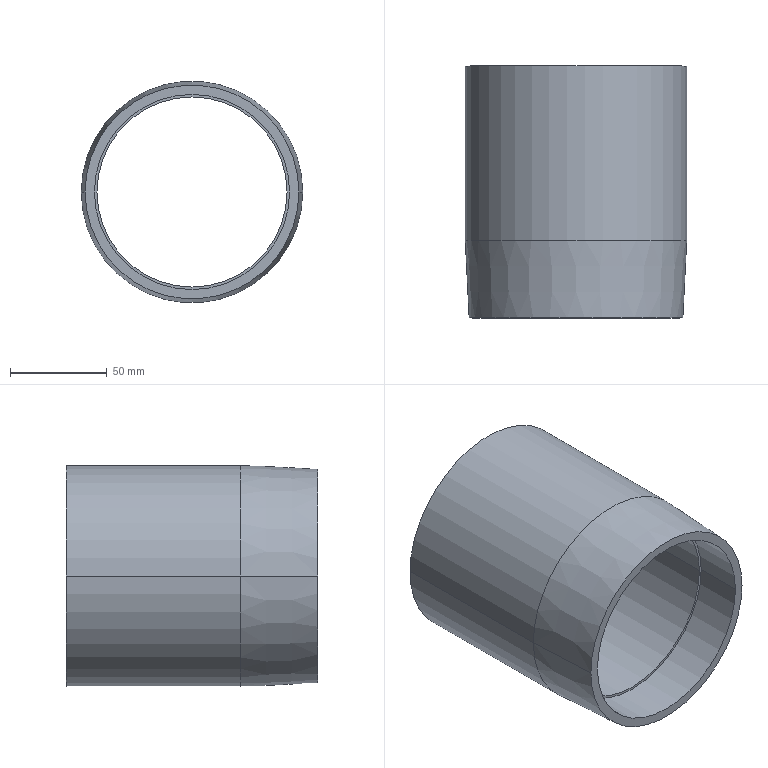Part | STEP file | ROLLER.2.stp | 1 solid | 14 faces | box 114.3 x 130 x 114.3 mm | volume 316826 mm3 | cylinder 8 | plane 4 | cone 2 | commonest cylinder face diameters 100.7 x4 98.1 x2 114.3 x2
STEP:
#1=CARTESIAN_POINT('',(0.,0.,0.));
#2=DIRECTION('',(0.,0.,1.));
#3=DIRECTION('',(1.,0.,0.));
#4=AXIS2_PLACEMENT_3D('',#1,#2,#3);
#5=CARTESIAN_POINT('',(49.05,40.,0.));
#6=VERTEX_POINT('',#5);
#7=CARTESIAN_POINT('',(-49.05,40.,0.));
#8=VERTEX_POINT('',#7);
#9=CARTESIAN_POINT('',(0.,40.,0.));
#10=DIRECTION('',(0.,1.,0.));
#11=DIRECTION('',(1.,0.,0.));
#12=AXIS2_PLACEMENT_3D('',#9,#10,#11);
#13=CIRCLE('',#12,49.05);
#14=CARTESIAN_POINT('',(49.7,40.,0.));
#15=DIRECTION('',(0.,1.,0.));
#16=DIRECTION('',(1.,0.,0.));
#17=AXIS2_PLACEMENT_3D('',#14,#15,#16);
#18=PLANE('',#17);
#19=CARTESIAN_POINT('',(-49.7,0.));
#20=DIRECTION('',(1.,0.));
#21=AXIS2_PLACEMENT_2D('',#19,#20);
#22=CIRCLE('',#21,49.05);
#23=(GEOMETRIC_REPRESENTATION_CONTEXT(2)PARAMETRIC_REPRESENTATION_CONTEXT()REPRESENTATION_CONTEXT('',''));
#24=DEFINITIONAL_REPRESENTATION('',(#22),#23);
#25=PCURVE('',#18,#24);
#26=CARTESIAN_POINT('',(0.,-2.5,0.));
#27=DIRECTION('',(0.,1.,0.));
#28=DIRECTION('',(1.,0.,0.));
#29=AXIS2_PLACEMENT_3D('',#26,#27,#28);
#30=CYLINDRICAL_SURFACE('',#29,49.05);
#31=CARTESIAN_POINT('',(0.,42.5));
#32=DIRECTION('',(1.,0.));
#33=VECTOR('',#32,1.);
#34=LINE('',#31,#33);
#35=(GEOMETRIC_REPRESENTATION_CONTEXT(2)PARAMETRIC_REPRESENTATION_CONTEXT()REPRESENTATION_CONTEXT('',''));
#36=DEFINITIONAL_REPRESENTATION('',(#34),#35);
#37=PCURVE('',#30,#36);
#38=SURFACE_CURVE('',#13,(#25,#37),.PCURVE_S1.);
#39=EDGE_CURVE('',#6,#8,#38,.T.);
#40=ORIENTED_EDGE('',*,*,#39,.F.);
#41=CARTESIAN_POINT('',(0.,40.,0.));
#42=DIRECTION('',(0.,1.,0.));
#43=DIRECTION('',(1.,0.,0.));
#44=AXIS2_PLACEMENT_3D('',#41,#42,#43);
#45=CIRCLE('',#44,49.05);
#46=CARTESIAN_POINT('',(-49.7,0.));
#47=DIRECTION('',(1.,0.));
#48=AXIS2_PLACEMENT_2D('',#46,#47);
#49=CIRCLE('',#48,49.05);
#50=(GEOMETRIC_REPRESENTATION_CONTEXT(2)PARAMETRIC_REPRESENTATION_CONTEXT()REPRESENTATION_CONTEXT('',''));
#51=DEFINITIONAL_REPRESENTATION('',(#49),#50);
#52=PCURVE('',#18,#51);
#53=CARTESIAN_POINT('',(0.,-2.5,0.));
#54=DIRECTION('',(0.,1.,0.));
#55=DIRECTION('',(1.,0.,0.));
#56=AXIS2_PLACEMENT_3D('',#53,#54,#55);
#57=CYLINDRICAL_SURFACE('',#56,49.05);
#58=CARTESIAN_POINT('',(0.,42.5));
#59=DIRECTION('',(1.,0.));
#60=VECTOR('',#59,1.);
#61=LINE('',#58,#60);
#62=(GEOMETRIC_REPRESENTATION_CONTEXT(2)PARAMETRIC_REPRESENTATION_CONTEXT()REPRESENTATION_CONTEXT('',''));
#63=DEFINITIONAL_REPRESENTATION('',(#61),#62);
#64=PCURVE('',#57,#63);
#65=SURFACE_CURVE('',#45,(#52,#64),.PCURVE_S1.);
#66=EDGE_CURVE('',#8,#6,#65,.T.);
#67=ORIENTED_EDGE('',*,*,#66,.F.);
#68=EDGE_LOOP('',(#40,#67));
#69=FACE_BOUND('',#68,.T.);
#70=CARTESIAN_POINT('',(50.35,40.,0.));
#71=VERTEX_POINT('',#70);
#72=CARTESIAN_POINT('',(-50.35,40.,0.));
#73=VERTEX_POINT('',#72);
#74=CARTESIAN_POINT('',(0.,40.,0.));
#75=DIRECTION('',(0.,1.,0.));
#76=DIRECTION('',(1.,0.,0.));
#77=AXIS2_PLACEMENT_3D('',#74,#75,#76);
#78=CIRCLE('',#77,50.35);
#79=CARTESIAN_POINT('',(-49.7,0.));
#80=DIRECTION('',(1.,0.));
#81=AXIS2_PLACEMENT_2D('',#79,#80);
#82=CIRCLE('',#81,50.35);
#83=(GEOMETRIC_REPRESENTATION_CONTEXT(2)PARAMETRIC_REPRESENTATION_CONTEXT()REPRESENTATION_CONTEXT('',''));
#84=DEFINITIONAL_REPRESENTATION('',(#82),#83);
#85=PCURVE('',#18,#84);
#86=CARTESIAN_POINT('',(0.,50.,0.));
#87=DIRECTION('',(0.,1.,0.));
#88=DIRECTION('',(1.,0.,0.));
#89=AXIS2_PLACEMENT_3D('',#86,#87,#88);
#90=CYLINDRICAL_SURFACE('',#89,50.35);
#91=CARTESIAN_POINT('',(0.,-10.));
#92=DIRECTION('',(1.,0.));
#93=VECTOR('',#92,1.);
#94=LINE('',#91,#93);
#95=(GEOMETRIC_REPRESENTATION_CONTEXT(2)PARAMETRIC_REPRESENTATION_CONTEXT()REPRESENTATION_CONTEXT('',''));
#96=DEFINITIONAL_REPRESENTATION('',(#94),#95);
#97=PCURVE('',#90,#96);
#98=SURFACE_CURVE('',#78,(#85,#97),.PCURVE_S1.);
#99=EDGE_CURVE('',#71,#73,#98,.T.);
#100=ORIENTED_EDGE('',*,*,#99,.T.);
#101=CARTESIAN_POINT('',(0.,40.,0.));
#102=DIRECTION('',(0.,1.,0.));
#103=DIRECTION('',(1.,0.,0.));
#104=AXIS2_PLACEMENT_3D('',#101,#102,#103);
#105=CIRCLE('',#104,50.35);
#106=CARTESIAN_POINT('',(-49.7,0.));
#107=DIRECTION('',(1.,0.));
#108=AXIS2_PLACEMENT_2D('',#106,#107);
#109=CIRCLE('',#108,50.35);
#110=(GEOMETRIC_REPRESENTATION_CONTEXT(2)PARAMETRIC_REPRESENTATION_CONTEXT()REPRESENTATION_CONTEXT('',''));
#111=DEFINITIONAL_REPRESENTATION('',(#109),#110);
#112=PCURVE('',#18,#111);
#113=CARTESIAN_POINT('',(0.,50.,0.));
#114=DIRECTION('',(0.,1.,0.));
#115=DIRECTION('',(1.,0.,0.));
#116=AXIS2_PLACEMENT_3D('',#113,#114,#115);
#117=CYLINDRICAL_SURFACE('',#116,50.35);
#118=CARTESIAN_POINT('',(0.,-10.));
#119=DIRECTION('',(1.,0.));
#120=VECTOR('',#119,1.);
#121=LINE('',#118,#120);
#122=(GEOMETRIC_REPRESENTATION_CONTEXT(2)PARAMETRIC_REPRESENTATION_CONTEXT()REPRESENTATION_CONTEXT('',''));
#123=DEFINITIONAL_REPRESENTATION('',(#121),#122);
#124=PCURVE('',#117,#123);
#125=SURFACE_CURVE('',#105,(#112,#124),.PCURVE_S1.);
#126=EDGE_CURVE('',#73,#71,#125,.T.);
#127=ORIENTED_EDGE('',*,*,#126,.T.);
#128=EDGE_LOOP('',(#100,#127));
#129=FACE_BOUND('',#128,.T.);
#130=ADVANCED_FACE('',(#69,#129),#18,.T.);
#131=CARTESIAN_POINT('',(50.35,65.,0.));
#132=VERTEX_POINT('',#131);
#133=CARTESIAN_POINT('',(-50.35,65.,0.));
#134=VERTEX_POINT('',#133);
#135=CARTESIAN_POINT('',(0.,65.,0.));
#136=DIRECTION('',(0.,1.,0.));
#137=DIRECTION('',(1.,0.,0.));
#138=AXIS2_PLACEMENT_3D('',#135,#136,#137);
#139=CIRCLE('',#138,50.35);
#140=CARTESIAN_POINT('',(53.75,65.,0.));
#141=DIRECTION('',(0.,1.,0.));
#142=DIRECTION('',(1.,0.,0.));
#143=AXIS2_PLACEMENT_3D('',#140,#141,#142);
#144=PLANE('',#143);
#145=CARTESIAN_POINT('',(-53.75,0.));
#146=DIRECTION('',(1.,0.));
#147=AXIS2_PLACEMENT_2D('',#145,#146);
#148=CIRCLE('',#147,50.35);
#149=(GEOMETRIC_REPRESENTATION_CONTEXT(2)PARAMETRIC_REPRESENTATION_CONTEXT()REPRESENTATION_CONTEXT('',''));
#150=DEFINITIONAL_REPRESENTATION('',(#148),#149);
#151=PCURVE('',#144,#150);
#152=CARTESIAN_POINT('',(0.,15.));
#153=DIRECTION('',(1.,0.));
#154=VECTOR('',#153,1.);
#155=LINE('',#152,#154);
#156=(GEOMETRIC_REPRESENTATION_CONTEXT(2)PARAMETRIC_REPRESENTATION_CONTEXT()REPRESENTATION_CONTEXT('',''));
#157=DEFINITIONAL_REPRESENTATION('',(#155),#156);
#158=PCURVE('',#90,#157);
#159=SURFACE_CURVE('',#139,(#151,#158),.PCURVE_S1.);
#160=EDGE_CURVE('',#132,#134,#159,.T.);
#161=ORIENTED_EDGE('',*,*,#160,.F.);
#162=CARTESIAN_POINT('',(0.,65.,0.));
#163=DIRECTION('',(0.,1.,0.));
#164=DIRECTION('',(1.,0.,0.));
#165=AXIS2_PLACEMENT_3D('',#162,#163,#164);
#166=CIRCLE('',#165,50.35);
#167=CARTESIAN_POINT('',(-53.75,0.));
#168=DIRECTION('',(1.,0.));
#169=AXIS2_PLACEMENT_2D('',#167,#168);
#170=CIRCLE('',#169,50.35);
#171=(GEOMETRIC_REPRESENTATION_CONTEXT(2)PARAMETRIC_REPRESENTATION_CONTEXT()REPRESENTATION_CONTEXT('',''));
#172=DEFINITIONAL_REPRESENTATION('',(#170),#171);
#173=PCURVE('',#144,#172);
#174=CARTESIAN_POINT('',(0.,15.));
#175=DIRECTION('',(1.,0.));
#176=VECTOR('',#175,1.);
#177=LINE('',#174,#176);
#178=(GEOMETRIC_REPRESENTATION_CONTEXT(2)PARAMETRIC_REPRESENTATION_CONTEXT()REPRESENTATION_CONTEXT('',''));
#179=DEFINITIONAL_REPRESENTATION('',(#177),#178);
#180=PCURVE('',#117,#179);
#181=SURFACE_CURVE('',#166,(#173,#180),.PCURVE_S1.);
#182=EDGE_CURVE('',#134,#132,#181,.T.);
#183=ORIENTED_EDGE('',*,*,#182,.F.);
#184=EDGE_LOOP('',(#161,#183));
#185=FACE_BOUND('',#184,.T.);
#186=CARTESIAN_POINT('',(57.15,65.,0.));
#187=VERTEX_POINT('',#186);
#188=CARTESIAN_POINT('',(-57.15,65.,0.));
#189=VERTEX_POINT('',#188);
#190=CARTESIAN_POINT('',(0.,65.,0.));
#191=DIRECTION('',(0.,1.,0.));
#192=DIRECTION('',(1.,0.,0.));
#193=AXIS2_PLACEMENT_3D('',#190,#191,#192);
#194=CIRCLE('',#193,57.15);
#195=CARTESIAN_POINT('',(-53.75,0.));
#196=DIRECTION('',(1.,0.));
#197=AXIS2_PLACEMENT_2D('',#195,#196);
#198=CIRCLE('',#197,57.15);
#199=(GEOMETRIC_REPRESENTATION_CONTEXT(2)PARAMETRIC_REPRESENTATION_CONTEXT()REPRESENTATION_CONTEXT('',''));
#200=DEFINITIONAL_REPRESENTATION('',(#198),#199);
#201=PCURVE('',#144,#200);
#202=CARTESIAN_POINT('',(0.,20.,0.));
#203=DIRECTION('',(0.,1.,0.));
#204=DIRECTION('',(1.,0.,0.));
#205=AXIS2_PLACEMENT_3D('',#202,#203,#204);
#206=CYLINDRICAL_SURFACE('',#205,57.15);
#207=CARTESIAN_POINT('',(0.,45.));
#208=DIRECTION('',(1.,0.));
#209=VECTOR('',#208,1.);
#210=LINE('',#207,#209);
#211=(GEOMETRIC_REPRESENTATION_CONTEXT(2)PARAMETRIC_REPRESENTATION_CONTEXT()REPRESENTATION_CONTEXT('',''));
#212=DEFINITIONAL_REPRESENTATION('',(#210),#211);
#213=PCURVE('',#206,#212);
#214=SURFACE_CURVE('',#194,(#201,#213),.PCURVE_S1.);
#215=EDGE_CURVE('',#187,#189,#214,.T.);
#216=ORIENTED_EDGE('',*,*,#215,.T.);
#217=CARTESIAN_POINT('',(0.,65.,0.));
#218=DIRECTION('',(0.,1.,0.));
#219=DIRECTION('',(1.,0.,0.));
#220=AXIS2_PLACEMENT_3D('',#217,#218,#219);
#221=CIRCLE('',#220,57.15);
#222=CARTESIAN_POINT('',(-53.75,0.));
#223=DIRECTION('',(1.,0.));
#224=AXIS2_PLACEMENT_2D('',#222,#223);
#225=CIRCLE('',#224,57.15);
#226=(GEOMETRIC_REPRESENTATION_CONTEXT(2)PARAMETRIC_REPRESENTATION_CONTEXT()REPRESENTATION_CONTEXT('',''));
#227=DEFINITIONAL_REPRESENTATION('',(#225),#226);
#228=PCURVE('',#144,#227);
#229=CARTESIAN_POINT('',(0.,20.,0.));
#230=DIRECTION('',(0.,1.,0.));
#231=DIRECTION('',(1.,0.,0.));
#232=AXIS2_PLACEMENT_3D('',#229,#230,#231);
#233=CYLINDRICAL_SURFACE('',#232,57.15);
#234=CARTESIAN_POINT('',(0.,45.));
#235=DIRECTION('',(1.,0.));
#236=VECTOR('',#235,1.);
#237=LINE('',#234,#236);
#238=(GEOMETRIC_REPRESENTATION_CONTEXT(2)PARAMETRIC_REPRESENTATION_CONTEXT()REPRESENTATION_CONTEXT('',''));
#239=DEFINITIONAL_REPRESENTATION('',(#237),#238);
#240=PCURVE('',#233,#239);
#241=SURFACE_CURVE('',#221,(#228,#240),.PCURVE_S1.);
#242=EDGE_CURVE('',#189,#187,#241,.T.);
#243=ORIENTED_EDGE('',*,*,#242,.T.);
#244=EDGE_LOOP('',(#216,#243));
#245=FACE_BOUND('',#244,.T.);
#246=ADVANCED_FACE('',(#185,#245),#144,.T.);
#247=CARTESIAN_POINT('',(57.15,-25.,0.));
#248=VERTEX_POINT('',#247);
#249=CARTESIAN_POINT('',(57.15,65.,0.));
#250=DIRECTION('',(0.,-1.,0.));
#251=VECTOR('',#250,1.);
#252=LINE('',#249,#251);
#253=CARTESIAN_POINT('',(0.,45.));
#254=DIRECTION('',(0.,-1.));
#255=VECTOR('',#254,1.);
#256=LINE('',#253,#255);
#257=(GEOMETRIC_REPRESENTATION_CONTEXT(2)PARAMETRIC_REPRESENTATION_CONTEXT()REPRESENTATION_CONTEXT('',''));
#258=DEFINITIONAL_REPRESENTATION('',(#256),#257);
#259=PCURVE('',#206,#258);
#260=CARTESIAN_POINT('',(6.283,45.));
#261=DIRECTION('',(0.,-1.));
#262=VECTOR('',#261,1.);
#263=LINE('',#260,#262);
#264=(GEOMETRIC_REPRESENTATION_CONTEXT(2)PARAMETRIC_REPRESENTATION_CONTEXT()REPRESENTATION_CONTEXT('',''));
#265=DEFINITIONAL_REPRESENTATION('',(#263),#264);
#266=PCURVE('',#233,#265);
#267=SURFACE_CURVE('',#252,(#259,#266),.PCURVE_S1.);
#268=EDGE_CURVE('',#187,#248,#267,.T.);
#269=ORIENTED_EDGE('',*,*,#268,.T.);
#270=CARTESIAN_POINT('',(-57.15,-25.,0.));
#271=VERTEX_POINT('',#270);
#272=CARTESIAN_POINT('',(0.,-25.,0.));
#273=DIRECTION('',(0.,1.,0.));
#274=DIRECTION('',(1.,0.,0.));
#275=AXIS2_PLACEMENT_3D('',#272,#273,#274);
#276=CIRCLE('',#275,57.15);
#277=CARTESIAN_POINT('',(0.,-45.));
#278=DIRECTION('',(1.,0.));
#279=VECTOR('',#278,1.);
#280=LINE('',#277,#279);
#281=(GEOMETRIC_REPRESENTATION_CONTEXT(2)PARAMETRIC_REPRESENTATION_CONTEXT()REPRESENTATION_CONTEXT('',''));
#282=DEFINITIONAL_REPRESENTATION('',(#280),#281);
#283=PCURVE('',#206,#282);
#284=CARTESIAN_POINT('',(0.,-45.,0.));
#285=DIRECTION('',(0.,1.,0.));
#286=DIRECTION('',(1.,0.,0.));
#287=AXIS2_PLACEMENT_3D('',#284,#285,#286);
#288=CONICAL_SURFACE('',#287,56.15,0.04996);
#289=CARTESIAN_POINT('',(0.,20.));
#290=DIRECTION('',(1.,0.));
#291=VECTOR('',#290,1.);
#292=LINE('',#289,#291);
#293=(GEOMETRIC_REPRESENTATION_CONTEXT(2)PARAMETRIC_REPRESENTATION_CONTEXT()REPRESENTATION_CONTEXT('',''));
#294=DEFINITIONAL_REPRESENTATION('',(#292),#293);
#295=PCURVE('',#288,#294);
#296=SURFACE_CURVE('',#276,(#283,#295),.PCURVE_S1.);
#297=EDGE_CURVE('',#248,#271,#296,.T.);
#298=ORIENTED_EDGE('',*,*,#297,.T.);
#299=CARTESIAN_POINT('',(-57.15,65.,0.));
#300=DIRECTION('',(0.,-1.,0.));
#301=VECTOR('',#300,1.);
#302=LINE('',#299,#301);
#303=CARTESIAN_POINT('',(3.142,45.));
#304=DIRECTION('',(0.,-1.));
#305=VECTOR('',#304,1.);
#306=LINE('',#303,#305);
#307=(GEOMETRIC_REPRESENTATION_CONTEXT(2)PARAMETRIC_REPRESENTATION_CONTEXT()REPRESENTATION_CONTEXT('',''));
#308=DEFINITIONAL_REPRESENTATION('',(#306),#307);
#309=PCURVE('',#206,#308);
#310=CARTESIAN_POINT('',(3.142,45.));
#311=DIRECTION('',(0.,-1.));
#312=VECTOR('',#311,1.);
#313=LINE('',#310,#312);
#314=(GEOMETRIC_REPRESENTATION_CONTEXT(2)PARAMETRIC_REPRESENTATION_CONTEXT()REPRESENTATION_CONTEXT('',''));
#315=DEFINITIONAL_REPRESENTATION('',(#313),#314);
#316=PCURVE('',#233,#315);
#317=SURFACE_CURVE('',#302,(#309,#316),.PCURVE_S1.);
#318=EDGE_CURVE('',#189,#271,#317,.T.);
#319=ORIENTED_EDGE('',*,*,#318,.F.);
#320=ORIENTED_EDGE('',*,*,#215,.F.);
#321=EDGE_LOOP('',(#269,#298,#319,#320));
#322=FACE_BOUND('',#321,.T.);
#323=ADVANCED_FACE('',(#322),#206,.T.);
#324=CARTESIAN_POINT('',(55.15,-65.,0.));
#325=VERTEX_POINT('',#324);
#326=CARTESIAN_POINT('',(57.15,-25.,0.));
#327=DIRECTION('',(-0.04994,-0.9988,0.));
#328=VECTOR('',#327,1.);
#329=LINE('',#326,#328);
#330=CARTESIAN_POINT('',(0.,20.));
#331=DIRECTION('',(0.,-1.));
#332=VECTOR('',#331,1.);
#333=LINE('',#330,#332);
#334=(GEOMETRIC_REPRESENTATION_CONTEXT(2)PARAMETRIC_REPRESENTATION_CONTEXT()REPRESENTATION_CONTEXT('',''));
#335=DEFINITIONAL_REPRESENTATION('',(#333),#334);
#336=PCURVE('',#288,#335);
#337=CARTESIAN_POINT('',(0.,-45.,0.));
#338=DIRECTION('',(0.,1.,0.));
#339=DIRECTION('',(1.,0.,0.));
#340=AXIS2_PLACEMENT_3D('',#337,#338,#339);
#341=CONICAL_SURFACE('',#340,56.15,0.04996);
#342=CARTESIAN_POINT('',(6.283,20.));
#343=DIRECTION('',(0.,-1.));
#344=VECTOR('',#343,1.);
#345=LINE('',#342,#344);
#346=(GEOMETRIC_REPRESENTATION_CONTEXT(2)PARAMETRIC_REPRESENTATION_CONTEXT()REPRESENTATION_CONTEXT('',''));
#347=DEFINITIONAL_REPRESENTATION('',(#345),#346);
#348=PCURVE('',#341,#347);
#349=SURFACE_CURVE('',#329,(#336,#348),.PCURVE_S1.);
#350=EDGE_CURVE('',#248,#325,#349,.T.);
#351=ORIENTED_EDGE('',*,*,#350,.T.);
#352=CARTESIAN_POINT('',(-55.15,-65.,0.));
#353=VERTEX_POINT('',#352);
#354=CARTESIAN_POINT('',(0.,-65.,0.));
#355=DIRECTION('',(0.,1.,0.));
#356=DIRECTION('',(1.,0.,0.));
#357=AXIS2_PLACEMENT_3D('',#354,#355,#356);
#358=CIRCLE('',#357,55.15);
#359=CARTESIAN_POINT('',(0.,-20.));
#360=DIRECTION('',(1.,0.));
#361=VECTOR('',#360,1.);
#362=LINE('',#359,#361);
#363=(GEOMETRIC_REPRESENTATION_CONTEXT(2)PARAMETRIC_REPRESENTATION_CONTEXT()REPRESENTATION_CONTEXT('',''));
#364=DEFINITIONAL_REPRESENTATION('',(#362),#363);
#365=PCURVE('',#288,#364);
#366=CARTESIAN_POINT('',(52.75,-65.,0.));
#367=DIRECTION('',(0.,-1.,0.));
#368=DIRECTION('',(0.,0.,-1.));
#369=AXIS2_PLACEMENT_3D('',#366,#367,#368);
#370=PLANE('',#369);
#371=CARTESIAN_POINT('',(0.,2.4));
#372=CARTESIAN_POINT('',(95.523,2.4));
#373=CARTESIAN_POINT('',(47.761,-80.325));
#374=CARTESIAN_POINT('',(0.,-163.05));
#375=CARTESIAN_POINT('',(-47.761,-80.325));
#376=CARTESIAN_POINT('',(-95.523,2.4));
#377=CARTESIAN_POINT('',(0.,2.4));
#378=(BOUNDED_CURVE()B_SPLINE_CURVE(2,(#371,#372,#373,#374,#375,#376,#377),.UNSPECIFIED.,.T.,.F.)B_SPLINE_CURVE_WITH_KNOTS((1,2,2,2,2,1),(-2.094,0.,2.094,4.189,6.283,8.378),.UNSPECIFIED.)CURVE()GEOMETRIC_REPRESENTATION_ITEM()RATIONAL_B_SPLINE_CURVE((1.,0.5,1.,0.5,1.,0.5,1.))REPRESENTATION_ITEM(''));
#379=(GEOMETRIC_REPRESENTATION_CONTEXT(2)PARAMETRIC_REPRESENTATION_CONTEXT()REPRESENTATION_CONTEXT('',''));
#380=DEFINITIONAL_REPRESENTATION('',(#378),#379);
#381=PCURVE('',#370,#380);
#382=SURFACE_CURVE('',#358,(#365,#381),.PCURVE_S1.);
#383=EDGE_CURVE('',#325,#353,#382,.T.);
#384=ORIENTED_EDGE('',*,*,#383,.T.);
#385=CARTESIAN_POINT('',(-57.15,-25.,0.));
#386=DIRECTION('',(0.04994,-0.9988,0.));
#387=VECTOR('',#386,1.);
#388=LINE('',#385,#387);
#389=CARTESIAN_POINT('',(3.142,20.));
#390=DIRECTION('',(0.,-1.));
#391=VECTOR('',#390,1.);
#392=LINE('',#389,#391);
#393=(GEOMETRIC_REPRESENTATION_CONTEXT(2)PARAMETRIC_REPRESENTATION_CONTEXT()REPRESENTATION_CONTEXT('',''));
#394=DEFINITIONAL_REPRESENTATION('',(#392),#393);
#395=PCURVE('',#288,#394);
#396=CARTESIAN_POINT('',(3.142,20.));
#397=DIRECTION('',(0.,-1.));
#398=VECTOR('',#397,1.);
#399=LINE('',#396,#398);
#400=(GEOMETRIC_REPRESENTATION_CONTEXT(2)PARAMETRIC_REPRESENTATION_CONTEXT()REPRESENTATION_CONTEXT('',''));
#401=DEFINITIONAL_REPRESENTATION('',(#399),#400);
#402=PCURVE('',#341,#401);
#403=SURFACE_CURVE('',#388,(#395,#402),.PCURVE_S1.);
#404=EDGE_CURVE('',#271,#353,#403,.T.);
#405=ORIENTED_EDGE('',*,*,#404,.F.);
#406=ORIENTED_EDGE('',*,*,#297,.F.);
#407=EDGE_LOOP('',(#351,#384,#405,#406));
#408=FACE_BOUND('',#407,.T.);
#409=ADVANCED_FACE('',(#408),#288,.T.);
#410=CARTESIAN_POINT('',(50.35,-65.,0.));
#411=VERTEX_POINT('',#410);
#412=CARTESIAN_POINT('',(-50.35,-65.,0.));
#413=VERTEX_POINT('',#412);
#414=CARTESIAN_POINT('',(0.,-65.,0.));
#415=DIRECTION('',(0.,1.,0.));
#416=DIRECTION('',(1.,0.,0.));
#417=AXIS2_PLACEMENT_3D('',#414,#415,#416);
#418=CIRCLE('',#417,50.35);
#419=CARTESIAN_POINT('',(0.,-2.4));
#420=CARTESIAN_POINT('',(87.209,-2.4));
#421=CARTESIAN_POINT('',(43.604,-77.925));
#422=CARTESIAN_POINT('',(0.,-153.45));
#423=CARTESIAN_POINT('',(-43.604,-77.925));
#424=CARTESIAN_POINT('',(-87.209,-2.4));
#425=CARTESIAN_POINT('',(0.,-2.4));
#426=(BOUNDED_CURVE()B_SPLINE_CURVE(2,(#419,#420,#421,#422,#423,#424,#425),.UNSPECIFIED.,.T.,.F.)B_SPLINE_CURVE_WITH_KNOTS((1,2,2,2,2,1),(-2.094,0.,2.094,4.189,6.283,8.378),.UNSPECIFIED.)CURVE()GEOMETRIC_REPRESENTATION_ITEM()RATIONAL_B_SPLINE_CURVE((1.,0.5,1.,0.5,1.,0.5,1.))REPRESENTATION_ITEM(''));
#427=(GEOMETRIC_REPRESENTATION_CONTEXT(2)PARAMETRIC_REPRESENTATION_CONTEXT()REPRESENTATION_CONTEXT('',''));
#428=DEFINITIONAL_REPRESENTATION('',(#426),#427);
#429=PCURVE('',#370,#428);
#430=CARTESIAN_POINT('',(0.,-52.5,0.));
#431=DIRECTION('',(0.,1.,0.));
#432=DIRECTION('',(1.,0.,0.));
#433=AXIS2_PLACEMENT_3D('',#430,#431,#432);
#434=CYLINDRICAL_SURFACE('',#433,50.35);
#435=CARTESIAN_POINT('',(0.,-12.5));
#436=DIRECTION('',(1.,0.));
#437=VECTOR('',#436,1.);
#438=LINE('',#435,#437);
#439=(GEOMETRIC_REPRESENTATION_CONTEXT(2)PARAMETRIC_REPRESENTATION_CONTEXT()REPRESENTATION_CONTEXT('',''));
#440=DEFINITIONAL_REPRESENTATION('',(#438),#439);
#441=PCURVE('',#434,#440);
#442=SURFACE_CURVE('',#418,(#429,#441),.PCURVE_S1.);
#443=EDGE_CURVE('',#411,#413,#442,.T.);
#444=ORIENTED_EDGE('',*,*,#443,.T.);
#445=CARTESIAN_POINT('',(0.,-65.,0.));
#446=DIRECTION('',(0.,1.,0.));
#447=DIRECTION('',(1.,0.,0.));
#448=AXIS2_PLACEMENT_3D('',#445,#446,#447);
#449=CIRCLE('',#448,50.35);
#450=CARTESIAN_POINT('',(0.,-2.4));
#451=CARTESIAN_POINT('',(87.209,-2.4));
#452=CARTESIAN_POINT('',(43.604,-77.925));
#453=CARTESIAN_POINT('',(0.,-153.45));
#454=CARTESIAN_POINT('',(-43.604,-77.925));
#455=CARTESIAN_POINT('',(-87.209,-2.4));
#456=CARTESIAN_POINT('',(0.,-2.4));
#457=(BOUNDED_CURVE()B_SPLINE_CURVE(2,(#450,#451,#452,#453,#454,#455,#456),.UNSPECIFIED.,.T.,.F.)B_SPLINE_CURVE_WITH_KNOTS((1,2,2,2,2,1),(-2.094,0.,2.094,4.189,6.283,8.378),.UNSPECIFIED.)CURVE()GEOMETRIC_REPRESENTATION_ITEM()RATIONAL_B_SPLINE_CURVE((1.,0.5,1.,0.5,1.,0.5,1.))REPRESENTATION_ITEM(''));
#458=(GEOMETRIC_REPRESENTATION_CONTEXT(2)PARAMETRIC_REPRESENTATION_CONTEXT()REPRESENTATION_CONTEXT('',''));
#459=DEFINITIONAL_REPRESENTATION('',(#457),#458);
#460=PCURVE('',#370,#459);
#461=CARTESIAN_POINT('',(0.,-52.5,0.));
#462=DIRECTION('',(0.,1.,0.));
#463=DIRECTION('',(1.,0.,0.));
#464=AXIS2_PLACEMENT_3D('',#461,#462,#463);
#465=CYLINDRICAL_SURFACE('',#464,50.35);
#466=CARTESIAN_POINT('',(0.,-12.5));
#467=DIRECTION('',(1.,0.));
#468=VECTOR('',#467,1.);
#469=LINE('',#466,#468);
#470=(GEOMETRIC_REPRESENTATION_CONTEXT(2)PARAMETRIC_REPRESENTATION_CONTEXT()REPRESENTATION_CONTEXT('',''));
#471=DEFINITIONAL_REPRESENTATION('',(#469),#470);
#472=PCURVE('',#465,#471);
#473=SURFACE_CURVE('',#449,(#460,#472),.PCURVE_S1.);
#474=EDGE_CURVE('',#413,#411,#473,.T.);
#475=ORIENTED_EDGE('',*,*,#474,.T.);
#476=EDGE_LOOP('',(#444,#475));
#477=FACE_BOUND('',#476,.T.);
#478=ORIENTED_EDGE('',*,*,#383,.F.);
#479=CARTESIAN_POINT('',(0.,-65.,0.));
#480=DIRECTION('',(0.,1.,0.));
#481=DIRECTION('',(1.,0.,0.));
#482=AXIS2_PLACEMENT_3D('',#479,#480,#481);
#483=CIRCLE('',#482,55.15);
#484=CARTESIAN_POINT('',(0.,2.4));
#485=CARTESIAN_POINT('',(95.523,2.4));
#486=CARTESIAN_POINT('',(47.761,-80.325));
#487=CARTESIAN_POINT('',(0.,-163.05));
#488=CARTESIAN_POINT('',(-47.761,-80.325));
#489=CARTESIAN_POINT('',(-95.523,2.4));
#490=CARTESIAN_POINT('',(0.,2.4));
#491=(BOUNDED_CURVE()B_SPLINE_CURVE(2,(#484,#485,#486,#487,#488,#489,#490),.UNSPECIFIED.,.T.,.F.)B_SPLINE_CURVE_WITH_KNOTS((1,2,2,2,2,1),(-2.094,0.,2.094,4.189,6.283,8.378),.UNSPECIFIED.)CURVE()GEOMETRIC_REPRESENTATION_ITEM()RATIONAL_B_SPLINE_CURVE((1.,0.5,1.,0.5,1.,0.5,1.))REPRESENTATION_ITEM(''));
#492=(GEOMETRIC_REPRESENTATION_CONTEXT(2)PARAMETRIC_REPRESENTATION_CONTEXT()REPRESENTATION_CONTEXT('',''));
#493=DEFINITIONAL_REPRESENTATION('',(#491),#492);
#494=PCURVE('',#370,#493);
#495=CARTESIAN_POINT('',(0.,-20.));
#496=DIRECTION('',(1.,0.));
#497=VECTOR('',#496,1.);
#498=LINE('',#495,#497);
#499=(GEOMETRIC_REPRESENTATION_CONTEXT(2)PARAMETRIC_REPRESENTATION_CONTEXT()REPRESENTATION_CONTEXT('',''));
#500=DEFINITIONAL_REPRESENTATION('',(#498),#499);
#501=PCURVE('',#341,#500);
#502=SURFACE_CURVE('',#483,(#494,#501),.PCURVE_S1.);
#503=EDGE_CURVE('',#353,#325,#502,.T.);
#504=ORIENTED_EDGE('',*,*,#503,.F.);
#505=EDGE_LOOP('',(#478,#504));
#506=FACE_BOUND('',#505,.T.);
#507=ADVANCED_FACE('',(#477,#506),#370,.T.);
#508=CARTESIAN_POINT('',(-50.35,-40.,0.));
#509=VERTEX_POINT('',#508);
#510=CARTESIAN_POINT('',(50.35,-40.,0.));
#511=VERTEX_POINT('',#510);
#512=CARTESIAN_POINT('',(0.,-40.,0.));
#513=DIRECTION('',(0.,1.,0.));
#514=DIRECTION('',(1.,0.,0.));
#515=AXIS2_PLACEMENT_3D('',#512,#513,#514);
#516=CIRCLE('',#515,50.35);
#517=CARTESIAN_POINT('',(0.,12.5));
#518=DIRECTION('',(1.,0.));
#519=VECTOR('',#518,1.);
#520=LINE('',#517,#519);
#521=(GEOMETRIC_REPRESENTATION_CONTEXT(2)PARAMETRIC_REPRESENTATION_CONTEXT()REPRESENTATION_CONTEXT('',''));
#522=DEFINITIONAL_REPRESENTATION('',(#520),#521);
#523=PCURVE('',#465,#522);
#524=CARTESIAN_POINT('',(49.7,-40.,0.));
#525=DIRECTION('',(0.,-1.,0.));
#526=DIRECTION('',(0.,0.,-1.));
#527=AXIS2_PLACEMENT_3D('',#524,#525,#526);
#528=PLANE('',#527);
#529=CARTESIAN_POINT('',(0.,0.65));
#530=CARTESIAN_POINT('',(87.209,0.65));
#531=CARTESIAN_POINT('',(43.604,-74.875));
#532=CARTESIAN_POINT('',(0.,-150.4));
#533=CARTESIAN_POINT('',(-43.604,-74.875));
#534=CARTESIAN_POINT('',(-87.209,0.65));
#535=CARTESIAN_POINT('',(0.,0.65));
#536=(BOUNDED_CURVE()B_SPLINE_CURVE(2,(#529,#530,#531,#532,#533,#534,#535),.UNSPECIFIED.,.T.,.F.)B_SPLINE_CURVE_WITH_KNOTS((1,2,2,2,2,1),(-2.094,0.,2.094,4.189,6.283,8.378),.UNSPECIFIED.)CURVE()GEOMETRIC_REPRESENTATION_ITEM()RATIONAL_B_SPLINE_CURVE((1.,0.5,1.,0.5,1.,0.5,1.))REPRESENTATION_ITEM(''));
#537=(GEOMETRIC_REPRESENTATION_CONTEXT(2)PARAMETRIC_REPRESENTATION_CONTEXT()REPRESENTATION_CONTEXT('',''));
#538=DEFINITIONAL_REPRESENTATION('',(#536),#537);
#539=PCURVE('',#528,#538);
#540=SURFACE_CURVE('',#516,(#523,#539),.PCURVE_S1.);
#541=EDGE_CURVE('',#509,#511,#540,.T.);
#542=ORIENTED_EDGE('',*,*,#541,.F.);
#543=CARTESIAN_POINT('',(-50.35,-40.,0.));
#544=DIRECTION('',(0.,-1.,0.));
#545=VECTOR('',#544,1.);
#546=LINE('',#543,#545);
#547=CARTESIAN_POINT('',(3.142,12.5));
#548=DIRECTION('',(0.,-1.));
#549=VECTOR('',#548,1.);
#550=LINE('',#547,#549);
#551=(GEOMETRIC_REPRESENTATION_CONTEXT(2)PARAMETRIC_REPRESENTATION_CONTEXT()REPRESENTATION_CONTEXT('',''));
#552=DEFINITIONAL_REPRESENTATION('',(#550),#551);
#553=PCURVE('',#465,#552);
#554=CARTESIAN_POINT('',(3.142,12.5));
#555=DIRECTION('',(0.,-1.));
#556=VECTOR('',#555,1.);
#557=LINE('',#554,#556);
#558=(GEOMETRIC_REPRESENTATION_CONTEXT(2)PARAMETRIC_REPRESENTATION_CONTEXT()REPRESENTATION_CONTEXT('',''));
#559=DEFINITIONAL_REPRESENTATION('',(#557),#558);
#560=PCURVE('',#434,#559);
#561=SURFACE_CURVE('',#546,(#553,#560),.PCURVE_S1.);
#562=EDGE_CURVE('',#509,#413,#561,.T.);
#563=ORIENTED_EDGE('',*,*,#562,.T.);
#564=ORIENTED_EDGE('',*,*,#474,.T.);
#565=CARTESIAN_POINT('',(50.35,-40.,0.));
#566=DIRECTION('',(0.,-1.,0.));
#567=VECTOR('',#566,1.);
#568=LINE('',#565,#567);
#569=CARTESIAN_POINT('',(6.283,12.5));
#570=DIRECTION('',(0.,-1.));
#571=VECTOR('',#570,1.);
#572=LINE('',#569,#571);
#573=(GEOMETRIC_REPRESENTATION_CONTEXT(2)PARAMETRIC_REPRESENTATION_CONTEXT()REPRESENTATION_CONTEXT('',''));
#574=DEFINITIONAL_REPRESENTATION('',(#572),#573);
#575=PCURVE('',#465,#574);
#576=CARTESIAN_POINT('',(0.,12.5));
#577=DIRECTION('',(0.,-1.));
#578=VECTOR('',#577,1.);
#579=LINE('',#576,#578);
#580=(GEOMETRIC_REPRESENTATION_CONTEXT(2)PARAMETRIC_REPRESENTATION_CONTEXT()REPRESENTATION_CONTEXT('',''));
#581=DEFINITIONAL_REPRESENTATION('',(#579),#580);
#582=PCURVE('',#434,#581);
#583=SURFACE_CURVE('',#568,(#575,#582),.PCURVE_S1.);
#584=EDGE_CURVE('',#511,#411,#583,.T.);
#585=ORIENTED_EDGE('',*,*,#584,.F.);
#586=EDGE_LOOP('',(#542,#563,#564,#585));
#587=FACE_BOUND('',#586,.F.);
#588=ADVANCED_FACE('',(#587),#465,.F.);
#589=CARTESIAN_POINT('',(49.05,-40.,0.));
#590=VERTEX_POINT('',#589);
#591=CARTESIAN_POINT('',(-49.05,-40.,0.));
#592=VERTEX_POINT('',#591);
#593=CARTESIAN_POINT('',(0.,-40.,0.));
#594=DIRECTION('',(0.,1.,0.));
#595=DIRECTION('',(1.,0.,0.));
#596=AXIS2_PLACEMENT_3D('',#593,#594,#595);
#597=CIRCLE('',#596,49.05);
#598=CARTESIAN_POINT('',(0.,-0.65));
#599=CARTESIAN_POINT('',(84.957,-0.65));
#600=CARTESIAN_POINT('',(42.479,-74.225));
#601=CARTESIAN_POINT('',(0.,-147.8));
#602=CARTESIAN_POINT('',(-42.479,-74.225));
#603=CARTESIAN_POINT('',(-84.957,-0.65));
#604=CARTESIAN_POINT('',(0.,-0.65));
#605=(BOUNDED_CURVE()B_SPLINE_CURVE(2,(#598,#599,#600,#601,#602,#603,#604),.UNSPECIFIED.,.T.,.F.)B_SPLINE_CURVE_WITH_KNOTS((1,2,2,2,2,1),(-2.094,0.,2.094,4.189,6.283,8.378),.UNSPECIFIED.)CURVE()GEOMETRIC_REPRESENTATION_ITEM()RATIONAL_B_SPLINE_CURVE((1.,0.5,1.,0.5,1.,0.5,1.))REPRESENTATION_ITEM(''));
#606=(GEOMETRIC_REPRESENTATION_CONTEXT(2)PARAMETRIC_REPRESENTATION_CONTEXT()REPRESENTATION_CONTEXT('',''));
#607=DEFINITIONAL_REPRESENTATION('',(#605),#606);
#608=PCURVE('',#528,#607);
#609=CARTESIAN_POINT('',(0.,-37.5));
#610=DIRECTION('',(1.,0.));
#611=VECTOR('',#610,1.);
#612=LINE('',#609,#611);
#613=(GEOMETRIC_REPRESENTATION_CONTEXT(2)PARAMETRIC_REPRESENTATION_CONTEXT()REPRESENTATION_CONTEXT('',''));
#614=DEFINITIONAL_REPRESENTATION('',(#612),#613);
#615=PCURVE('',#30,#614);
#616=SURFACE_CURVE('',#597,(#608,#615),.PCURVE_S1.);
#617=EDGE_CURVE('',#590,#592,#616,.T.);
#618=ORIENTED_EDGE('',*,*,#617,.T.);
#619=CARTESIAN_POINT('',(0.,-40.,0.));
#620=DIRECTION('',(0.,1.,0.));
#621=DIRECTION('',(1.,0.,0.));
#622=AXIS2_PLACEMENT_3D('',#619,#620,#621);
#623=CIRCLE('',#622,49.05);
#624=CARTESIAN_POINT('',(0.,-0.65));
#625=CARTESIAN_POINT('',(84.957,-0.65));
#626=CARTESIAN_POINT('',(42.479,-74.225));
#627=CARTESIAN_POINT('',(0.,-147.8));
#628=CARTESIAN_POINT('',(-42.479,-74.225));
#629=CARTESIAN_POINT('',(-84.957,-0.65));
#630=CARTESIAN_POINT('',(0.,-0.65));
#631=(BOUNDED_CURVE()B_SPLINE_CURVE(2,(#624,#625,#626,#627,#628,#629,#630),.UNSPECIFIED.,.T.,.F.)B_SPLINE_CURVE_WITH_KNOTS((1,2,2,2,2,1),(-2.094,0.,2.094,4.189,6.283,8.378),.UNSPECIFIED.)CURVE()GEOMETRIC_REPRESENTATION_ITEM()RATIONAL_B_SPLINE_CURVE((1.,0.5,1.,0.5,1.,0.5,1.))REPRESENTATION_ITEM(''));
#632=(GEOMETRIC_REPRESENTATION_CONTEXT(2)PARAMETRIC_REPRESENTATION_CONTEXT()REPRESENTATION_CONTEXT('',''));
#633=DEFINITIONAL_REPRESENTATION('',(#631),#632);
#634=PCURVE('',#528,#633);
#635=CARTESIAN_POINT('',(0.,-37.5));
#636=DIRECTION('',(1.,0.));
#637=VECTOR('',#636,1.);
#638=LINE('',#635,#637);
#639=(GEOMETRIC_REPRESENTATION_CONTEXT(2)PARAMETRIC_REPRESENTATION_CONTEXT()REPRESENTATION_CONTEXT('',''));
#640=DEFINITIONAL_REPRESENTATION('',(#638),#639);
#641=PCURVE('',#57,#640);
#642=SURFACE_CURVE('',#623,(#634,#641),.PCURVE_S1.);
#643=EDGE_CURVE('',#592,#590,#642,.T.);
#644=ORIENTED_EDGE('',*,*,#643,.T.);
#645=EDGE_LOOP('',(#618,#644));
#646=FACE_BOUND('',#645,.T.);
#647=CARTESIAN_POINT('',(0.,-40.,0.));
#648=DIRECTION('',(0.,1.,0.));
#649=DIRECTION('',(1.,0.,0.));
#650=AXIS2_PLACEMENT_3D('',#647,#648,#649);
#651=CIRCLE('',#650,50.35);
#652=CARTESIAN_POINT('',(0.,0.65));
#653=CARTESIAN_POINT('',(87.209,0.65));
#654=CARTESIAN_POINT('',(43.604,-74.875));
#655=CARTESIAN_POINT('',(0.,-150.4));
#656=CARTESIAN_POINT('',(-43.604,-74.875));
#657=CARTESIAN_POINT('',(-87.209,0.65));
#658=CARTESIAN_POINT('',(0.,0.65));
#659=(BOUNDED_CURVE()B_SPLINE_CURVE(2,(#652,#653,#654,#655,#656,#657,#658),.UNSPECIFIED.,.T.,.F.)B_SPLINE_CURVE_WITH_KNOTS((1,2,2,2,2,1),(-2.094,0.,2.094,4.189,6.283,8.378),.UNSPECIFIED.)CURVE()GEOMETRIC_REPRESENTATION_ITEM()RATIONAL_B_SPLINE_CURVE((1.,0.5,1.,0.5,1.,0.5,1.))REPRESENTATION_ITEM(''));
#660=(GEOMETRIC_REPRESENTATION_CONTEXT(2)PARAMETRIC_REPRESENTATION_CONTEXT()REPRESENTATION_CONTEXT('',''));
#661=DEFINITIONAL_REPRESENTATION('',(#659),#660);
#662=PCURVE('',#528,#661);
#663=CARTESIAN_POINT('',(0.,12.5));
#664=DIRECTION('',(1.,0.));
#665=VECTOR('',#664,1.);
#666=LINE('',#663,#665);
#667=(GEOMETRIC_REPRESENTATION_CONTEXT(2)PARAMETRIC_REPRESENTATION_CONTEXT()REPRESENTATION_CONTEXT('',''));
#668=DEFINITIONAL_REPRESENTATION('',(#666),#667);
#669=PCURVE('',#434,#668);
#670=SURFACE_CURVE('',#651,(#662,#669),.PCURVE_S1.);
#671=EDGE_CURVE('',#511,#509,#670,.T.);
#672=ORIENTED_EDGE('',*,*,#671,.F.);
#673=ORIENTED_EDGE('',*,*,#541,.F.);
#674=EDGE_LOOP('',(#672,#673));
#675=FACE_BOUND('',#674,.T.);
#676=ADVANCED_FACE('',(#646,#675),#528,.T.);
#677=ORIENTED_EDGE('',*,*,#66,.F.);
#678=CARTESIAN_POINT('',(-49.05,40.,0.));
#679=DIRECTION('',(0.,-1.,0.));
#680=VECTOR('',#679,1.);
#681=LINE('',#678,#680);
#682=CARTESIAN_POINT('',(3.142,42.5));
#683=DIRECTION('',(0.,-1.));
#684=VECTOR('',#683,1.);
#685=LINE('',#682,#684);
#686=(GEOMETRIC_REPRESENTATION_CONTEXT(2)PARAMETRIC_REPRESENTATION_CONTEXT()REPRESENTATION_CONTEXT('',''));
#687=DEFINITIONAL_REPRESENTATION('',(#685),#686);
#688=PCURVE('',#57,#687);
#689=CARTESIAN_POINT('',(3.142,42.5));
#690=DIRECTION('',(0.,-1.));
#691=VECTOR('',#690,1.);
#692=LINE('',#689,#691);
#693=(GEOMETRIC_REPRESENTATION_CONTEXT(2)PARAMETRIC_REPRESENTATION_CONTEXT()REPRESENTATION_CONTEXT('',''));
#694=DEFINITIONAL_REPRESENTATION('',(#692),#693);
#695=PCURVE('',#30,#694);
#696=SURFACE_CURVE('',#681,(#688,#695),.PCURVE_S1.);
#697=EDGE_CURVE('',#8,#592,#696,.T.);
#698=ORIENTED_EDGE('',*,*,#697,.T.);
#699=ORIENTED_EDGE('',*,*,#643,.T.);
#700=CARTESIAN_POINT('',(49.05,40.,0.));
#701=DIRECTION('',(0.,-1.,0.));
#702=VECTOR('',#701,1.);
#703=LINE('',#700,#702);
#704=CARTESIAN_POINT('',(6.283,42.5));
#705=DIRECTION('',(0.,-1.));
#706=VECTOR('',#705,1.);
#707=LINE('',#704,#706);
#708=(GEOMETRIC_REPRESENTATION_CONTEXT(2)PARAMETRIC_REPRESENTATION_CONTEXT()REPRESENTATION_CONTEXT('',''));
#709=DEFINITIONAL_REPRESENTATION('',(#707),#708);
#710=PCURVE('',#57,#709);
#711=CARTESIAN_POINT('',(0.,42.5));
#712=DIRECTION('',(0.,-1.));
#713=VECTOR('',#712,1.);
#714=LINE('',#711,#713);
#715=(GEOMETRIC_REPRESENTATION_CONTEXT(2)PARAMETRIC_REPRESENTATION_CONTEXT()REPRESENTATION_CONTEXT('',''));
#716=DEFINITIONAL_REPRESENTATION('',(#714),#715);
#717=PCURVE('',#30,#716);
#718=SURFACE_CURVE('',#703,(#710,#717),.PCURVE_S1.);
#719=EDGE_CURVE('',#6,#590,#718,.T.);
#720=ORIENTED_EDGE('',*,*,#719,.F.);
#721=EDGE_LOOP('',(#677,#698,#699,#720));
#722=FACE_BOUND('',#721,.F.);
#723=ADVANCED_FACE('',(#722),#57,.F.);
#724=ORIENTED_EDGE('',*,*,#182,.F.);
#725=CARTESIAN_POINT('',(-50.35,65.,0.));
#726=DIRECTION('',(0.,-1.,0.));
#727=VECTOR('',#726,1.);
#728=LINE('',#725,#727);
#729=CARTESIAN_POINT('',(3.142,15.));
#730=DIRECTION('',(0.,-1.));
#731=VECTOR('',#730,1.);
#732=LINE('',#729,#731);
#733=(GEOMETRIC_REPRESENTATION_CONTEXT(2)PARAMETRIC_REPRESENTATION_CONTEXT()REPRESENTATION_CONTEXT('',''));
#734=DEFINITIONAL_REPRESENTATION('',(#732),#733);
#735=PCURVE('',#117,#734);
#736=CARTESIAN_POINT('',(3.142,15.));
#737=DIRECTION('',(0.,-1.));
#738=VECTOR('',#737,1.);
#739=LINE('',#736,#738);
#740=(GEOMETRIC_REPRESENTATION_CONTEXT(2)PARAMETRIC_REPRESENTATION_CONTEXT()REPRESENTATION_CONTEXT('',''));
#741=DEFINITIONAL_REPRESENTATION('',(#739),#740);
#742=PCURVE('',#90,#741);
#743=SURFACE_CURVE('',#728,(#735,#742),.PCURVE_S1.);
#744=EDGE_CURVE('',#134,#73,#743,.T.);
#745=ORIENTED_EDGE('',*,*,#744,.T.);
#746=ORIENTED_EDGE('',*,*,#126,.T.);
#747=CARTESIAN_POINT('',(50.35,65.,0.));
#748=DIRECTION('',(0.,-1.,0.));
#749=VECTOR('',#748,1.);
#750=LINE('',#747,#749);
#751=CARTESIAN_POINT('',(6.283,15.));
#752=DIRECTION('',(0.,-1.));
#753=VECTOR('',#752,1.);
#754=LINE('',#751,#753);
#755=(GEOMETRIC_REPRESENTATION_CONTEXT(2)PARAMETRIC_REPRESENTATION_CONTEXT()REPRESENTATION_CONTEXT('',''));
#756=DEFINITIONAL_REPRESENTATION('',(#754),#755);
#757=PCURVE('',#117,#756);
#758=CARTESIAN_POINT('',(0.,15.));
#759=DIRECTION('',(0.,-1.));
#760=VECTOR('',#759,1.);
#761=LINE('',#758,#760);
#762=(GEOMETRIC_REPRESENTATION_CONTEXT(2)PARAMETRIC_REPRESENTATION_CONTEXT()REPRESENTATION_CONTEXT('',''));
#763=DEFINITIONAL_REPRESENTATION('',(#761),#762);
#764=PCURVE('',#90,#763);
#765=SURFACE_CURVE('',#750,(#757,#764),.PCURVE_S1.);
#766=EDGE_CURVE('',#132,#71,#765,.T.);
#767=ORIENTED_EDGE('',*,*,#766,.F.);
#768=EDGE_LOOP('',(#724,#745,#746,#767));
#769=FACE_BOUND('',#768,.F.);
#770=ADVANCED_FACE('',(#769),#117,.F.);
#771=ORIENTED_EDGE('',*,*,#99,.T.);
#772=ORIENTED_EDGE('',*,*,#744,.F.);
#773=ORIENTED_EDGE('',*,*,#160,.F.);
#774=ORIENTED_EDGE('',*,*,#766,.T.);
#775=EDGE_LOOP('',(#771,#772,#773,#774));
#776=FACE_BOUND('',#775,.F.);
#777=ADVANCED_FACE('',(#776),#90,.F.);
#778=ORIENTED_EDGE('',*,*,#617,.T.);
#779=ORIENTED_EDGE('',*,*,#697,.F.);
#780=ORIENTED_EDGE('',*,*,#39,.F.);
#781=ORIENTED_EDGE('',*,*,#719,.T.);
#782=EDGE_LOOP('',(#778,#779,#780,#781));
#783=FACE_BOUND('',#782,.F.);
#784=ADVANCED_FACE('',(#783),#30,.F.);
#785=ORIENTED_EDGE('',*,*,#443,.T.);
#786=ORIENTED_EDGE('',*,*,#562,.F.);
#787=ORIENTED_EDGE('',*,*,#671,.F.);
#788=ORIENTED_EDGE('',*,*,#584,.T.);
#789=EDGE_LOOP('',(#785,#786,#787,#788));
#790=FACE_BOUND('',#789,.F.);
#791=ADVANCED_FACE('',(#790),#434,.F.);
#792=ORIENTED_EDGE('',*,*,#350,.F.);
#793=CARTESIAN_POINT('',(0.,-25.,0.));
#794=DIRECTION('',(0.,1.,0.));
#795=DIRECTION('',(1.,0.,0.));
#796=AXIS2_PLACEMENT_3D('',#793,#794,#795);
#797=CIRCLE('',#796,57.15);
#798=CARTESIAN_POINT('',(0.,20.));
#799=DIRECTION('',(1.,0.));
#800=VECTOR('',#799,1.);
#801=LINE('',#798,#800);
#802=(GEOMETRIC_REPRESENTATION_CONTEXT(2)PARAMETRIC_REPRESENTATION_CONTEXT()REPRESENTATION_CONTEXT('',''));
#803=DEFINITIONAL_REPRESENTATION('',(#801),#802);
#804=PCURVE('',#341,#803);
#805=CARTESIAN_POINT('',(0.,-45.));
#806=DIRECTION('',(1.,0.));
#807=VECTOR('',#806,1.);
#808=LINE('',#805,#807);
#809=(GEOMETRIC_REPRESENTATION_CONTEXT(2)PARAMETRIC_REPRESENTATION_CONTEXT()REPRESENTATION_CONTEXT('',''));
#810=DEFINITIONAL_REPRESENTATION('',(#808),#809);
#811=PCURVE('',#233,#810);
#812=SURFACE_CURVE('',#797,(#804,#811),.PCURVE_S1.);
#813=EDGE_CURVE('',#271,#248,#812,.T.);
#814=ORIENTED_EDGE('',*,*,#813,.F.);
#815=ORIENTED_EDGE('',*,*,#404,.T.);
#816=ORIENTED_EDGE('',*,*,#503,.T.);
#817=EDGE_LOOP('',(#792,#814,#815,#816));
#818=FACE_BOUND('',#817,.T.);
#819=ADVANCED_FACE('',(#818),#341,.T.);
#820=ORIENTED_EDGE('',*,*,#268,.F.);
#821=ORIENTED_EDGE('',*,*,#242,.F.);
#822=ORIENTED_EDGE('',*,*,#318,.T.);
#823=ORIENTED_EDGE('',*,*,#813,.T.);
#824=EDGE_LOOP('',(#820,#821,#822,#823));
#825=FACE_BOUND('',#824,.T.);
#826=ADVANCED_FACE('',(#825),#233,.T.);
#827=CLOSED_SHELL('',(#130,#246,#323,#409,#507,#588,#676,#723,#770,#777,#784,#791,#819,#826));
#828=MANIFOLD_SOLID_BREP('',#827);
#829=(LENGTH_UNIT()NAMED_UNIT(*)SI_UNIT(.MILLI.,.METRE.));
#830=UNCERTAINTY_MEASURE_WITH_UNIT(LENGTH_MEASURE(0.0000001),#829,'','');
#831=(NAMED_UNIT(*)PLANE_ANGLE_UNIT()SI_UNIT($,.RADIAN.));
#832=(NAMED_UNIT(*)SI_UNIT($,.STERADIAN.)SOLID_ANGLE_UNIT());
#833=(GEOMETRIC_REPRESENTATION_CONTEXT(3)GLOBAL_UNCERTAINTY_ASSIGNED_CONTEXT((#830))GLOBAL_UNIT_ASSIGNED_CONTEXT((#829,#831,#832))REPRESENTATION_CONTEXT('',''));
#834=ADVANCED_BREP_SHAPE_REPRESENTATION('',(#4,#828),#833);